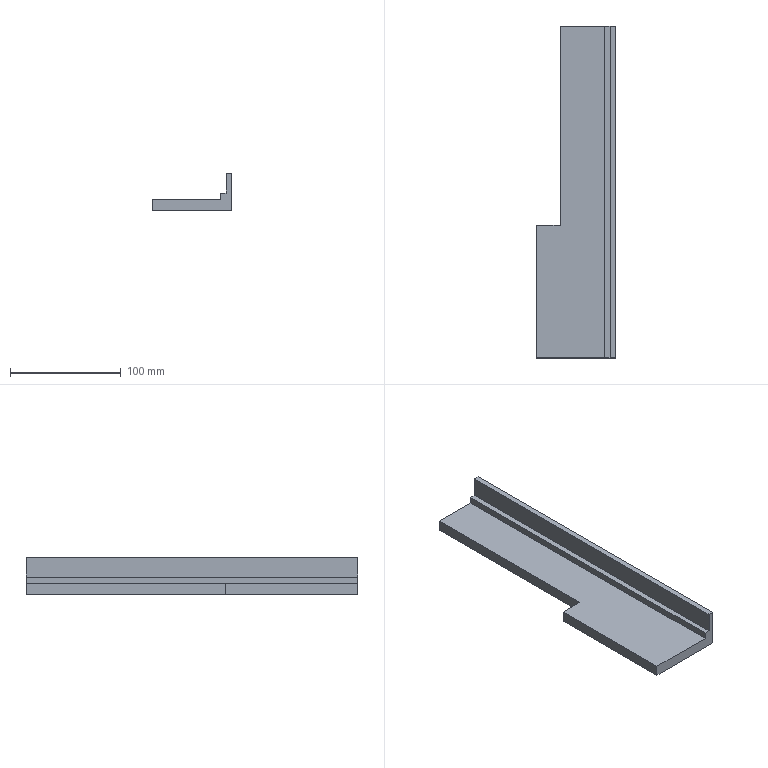Part | STEP file | Platform 1 slider plate 2 | 1 solid | 12 faces | box 71.5 x 300 x 34 mm | volume 220800 mm3 | plane 12
STEP:
#1=CARTESIAN_POINT('',(0.,150.,0.));
#2=VERTEX_POINT('',#1);
#3=CARTESIAN_POINT('',(0.,-30.,0.));
#4=VERTEX_POINT('',#3);
#5=CARTESIAN_POINT('',(0.,150.,0.));
#6=DIRECTION('',(0.,-1.,0.));
#7=VECTOR('',#6,1000.);
#8=LINE('',#5,#7);
#9=EDGE_CURVE('',#2,#4,#8,.T.);
#10=ORIENTED_EDGE('',*,*,#9,.T.);
#11=CARTESIAN_POINT('',(0.,-30.,10.));
#12=VERTEX_POINT('',#11);
#13=CARTESIAN_POINT('',(0.,-30.,-121.911));
#14=DIRECTION('',(0.,0.,1.));
#15=VECTOR('',#14,1000.);
#16=LINE('',#13,#15);
#17=EDGE_CURVE('',#4,#12,#16,.T.);
#18=ORIENTED_EDGE('',*,*,#17,.T.);
#19=CARTESIAN_POINT('',(0.,150.,10.));
#20=VERTEX_POINT('',#19);
#21=CARTESIAN_POINT('',(0.,150.,10.));
#22=DIRECTION('',(0.,-1.,0.));
#23=VECTOR('',#22,1000.);
#24=LINE('',#21,#23);
#25=EDGE_CURVE('',#20,#12,#24,.T.);
#26=ORIENTED_EDGE('',*,*,#25,.F.);
#27=CARTESIAN_POINT('',(0.,150.,10.));
#28=DIRECTION('',(0.,0.,1.));
#29=VECTOR('',#28,1000.);
#30=LINE('',#27,#29);
#31=EDGE_CURVE('',#2,#20,#30,.T.);
#32=ORIENTED_EDGE('',*,*,#31,.F.);
#33=EDGE_LOOP('',(#10,#18,#26,#32));
#34=FACE_OUTER_BOUND('',#33,.T.);
#35=CARTESIAN_POINT('',(0.,150.,10.));
#36=DIRECTION('',(1.,0.,0.));
#37=DIRECTION('',(0.,0.,-1.));
#38=AXIS2_PLACEMENT_3D('',#35,#36,#37);
#39=PLANE('',#38);
#40=ADVANCED_FACE('',(#34),#39,.F.);
#41=CARTESIAN_POINT('',(-21.5,-150.,10.));
#42=VERTEX_POINT('',#41);
#43=CARTESIAN_POINT('',(40.,-150.,10.));
#44=VERTEX_POINT('',#43);
#45=CARTESIAN_POINT('',(40.,-150.,10.));
#46=DIRECTION('',(1.,0.,0.));
#47=VECTOR('',#46,1000.);
#48=LINE('',#45,#47);
#49=EDGE_CURVE('',#42,#44,#48,.T.);
#50=ORIENTED_EDGE('',*,*,#49,.T.);
#51=CARTESIAN_POINT('',(40.,150.,10.));
#52=VERTEX_POINT('',#51);
#53=CARTESIAN_POINT('',(40.,150.,10.));
#54=DIRECTION('',(0.,-1.,0.));
#55=VECTOR('',#54,1000.);
#56=LINE('',#53,#55);
#57=EDGE_CURVE('',#52,#44,#56,.T.);
#58=ORIENTED_EDGE('',*,*,#57,.F.);
#59=CARTESIAN_POINT('',(40.,150.,10.));
#60=DIRECTION('',(1.,0.,0.));
#61=VECTOR('',#60,1000.);
#62=LINE('',#59,#61);
#63=EDGE_CURVE('',#20,#52,#62,.T.);
#64=ORIENTED_EDGE('',*,*,#63,.F.);
#65=ORIENTED_EDGE('',*,*,#25,.T.);
#66=CARTESIAN_POINT('',(-21.5,-30.,10.));
#67=VERTEX_POINT('',#66);
#68=CARTESIAN_POINT('',(0.,-30.,10.));
#69=DIRECTION('',(-1.,0.,0.));
#70=VECTOR('',#69,1000.);
#71=LINE('',#68,#70);
#72=EDGE_CURVE('',#12,#67,#71,.T.);
#73=ORIENTED_EDGE('',*,*,#72,.T.);
#74=CARTESIAN_POINT('',(-21.5,-150.,10.));
#75=DIRECTION('',(0.,-1.,0.));
#76=VECTOR('',#75,1000.);
#77=LINE('',#74,#76);
#78=EDGE_CURVE('',#67,#42,#77,.T.);
#79=ORIENTED_EDGE('',*,*,#78,.T.);
#80=EDGE_LOOP('',(#50,#58,#64,#65,#73,#79));
#81=FACE_OUTER_BOUND('',#80,.T.);
#82=CARTESIAN_POINT('',(40.,150.,10.));
#83=DIRECTION('',(0.,0.,-1.));
#84=DIRECTION('',(-1.,0.,0.));
#85=AXIS2_PLACEMENT_3D('',#82,#83,#84);
#86=PLANE('',#85);
#87=ADVANCED_FACE('',(#81),#86,.F.);
#88=CARTESIAN_POINT('',(40.,-150.,16.));
#89=VERTEX_POINT('',#88);
#90=CARTESIAN_POINT('',(40.,-150.,34.));
#91=DIRECTION('',(0.,0.,1.));
#92=VECTOR('',#91,1000.);
#93=LINE('',#90,#92);
#94=EDGE_CURVE('',#44,#89,#93,.T.);
#95=ORIENTED_EDGE('',*,*,#94,.T.);
#96=CARTESIAN_POINT('',(40.,150.,16.));
#97=VERTEX_POINT('',#96);
#98=CARTESIAN_POINT('',(40.,150.,16.));
#99=DIRECTION('',(0.,-1.,0.));
#100=VECTOR('',#99,1000.);
#101=LINE('',#98,#100);
#102=EDGE_CURVE('',#97,#89,#101,.T.);
#103=ORIENTED_EDGE('',*,*,#102,.F.);
#104=CARTESIAN_POINT('',(40.,150.,34.));
#105=DIRECTION('',(0.,0.,1.));
#106=VECTOR('',#105,1000.);
#107=LINE('',#104,#106);
#108=EDGE_CURVE('',#52,#97,#107,.T.);
#109=ORIENTED_EDGE('',*,*,#108,.F.);
#110=ORIENTED_EDGE('',*,*,#57,.T.);
#111=EDGE_LOOP('',(#95,#103,#109,#110));
#112=FACE_OUTER_BOUND('',#111,.T.);
#113=CARTESIAN_POINT('',(40.,150.,34.));
#114=DIRECTION('',(1.,0.,0.));
#115=DIRECTION('',(0.,0.,-1.));
#116=AXIS2_PLACEMENT_3D('',#113,#114,#115);
#117=PLANE('',#116);
#118=ADVANCED_FACE('',(#112),#117,.F.);
#119=CARTESIAN_POINT('',(45.,150.,34.));
#120=VERTEX_POINT('',#119);
#121=CARTESIAN_POINT('',(50.,150.,34.));
#122=VERTEX_POINT('',#121);
#123=CARTESIAN_POINT('',(50.,150.,34.));
#124=DIRECTION('',(1.,0.,0.));
#125=VECTOR('',#124,1000.);
#126=LINE('',#123,#125);
#127=EDGE_CURVE('',#120,#122,#126,.T.);
#128=ORIENTED_EDGE('',*,*,#127,.F.);
#129=CARTESIAN_POINT('',(45.,-150.,34.));
#130=VERTEX_POINT('',#129);
#131=CARTESIAN_POINT('',(45.,150.,34.));
#132=DIRECTION('',(0.,-1.,0.));
#133=VECTOR('',#132,1000.);
#134=LINE('',#131,#133);
#135=EDGE_CURVE('',#120,#130,#134,.T.);
#136=ORIENTED_EDGE('',*,*,#135,.T.);
#137=CARTESIAN_POINT('',(50.,-150.,34.));
#138=VERTEX_POINT('',#137);
#139=CARTESIAN_POINT('',(50.,-150.,34.));
#140=DIRECTION('',(1.,0.,0.));
#141=VECTOR('',#140,1000.);
#142=LINE('',#139,#141);
#143=EDGE_CURVE('',#130,#138,#142,.T.);
#144=ORIENTED_EDGE('',*,*,#143,.T.);
#145=CARTESIAN_POINT('',(50.,150.,34.));
#146=DIRECTION('',(0.,-1.,0.));
#147=VECTOR('',#146,1000.);
#148=LINE('',#145,#147);
#149=EDGE_CURVE('',#122,#138,#148,.T.);
#150=ORIENTED_EDGE('',*,*,#149,.F.);
#151=EDGE_LOOP('',(#128,#136,#144,#150));
#152=FACE_OUTER_BOUND('',#151,.T.);
#153=CARTESIAN_POINT('',(50.,150.,34.));
#154=DIRECTION('',(0.,0.,-1.));
#155=DIRECTION('',(-1.,0.,0.));
#156=AXIS2_PLACEMENT_3D('',#153,#154,#155);
#157=PLANE('',#156);
#158=ADVANCED_FACE('',(#152),#157,.F.);
#159=CARTESIAN_POINT('',(50.,-150.,0.));
#160=VERTEX_POINT('',#159);
#161=CARTESIAN_POINT('',(50.,-150.,0.));
#162=DIRECTION('',(0.,0.,-1.));
#163=VECTOR('',#162,1000.);
#164=LINE('',#161,#163);
#165=EDGE_CURVE('',#138,#160,#164,.T.);
#166=ORIENTED_EDGE('',*,*,#165,.T.);
#167=CARTESIAN_POINT('',(50.,150.,0.));
#168=VERTEX_POINT('',#167);
#169=CARTESIAN_POINT('',(50.,150.,0.));
#170=DIRECTION('',(0.,-1.,0.));
#171=VECTOR('',#170,1000.);
#172=LINE('',#169,#171);
#173=EDGE_CURVE('',#168,#160,#172,.T.);
#174=ORIENTED_EDGE('',*,*,#173,.F.);
#175=CARTESIAN_POINT('',(50.,150.,0.));
#176=DIRECTION('',(0.,0.,-1.));
#177=VECTOR('',#176,1000.);
#178=LINE('',#175,#177);
#179=EDGE_CURVE('',#122,#168,#178,.T.);
#180=ORIENTED_EDGE('',*,*,#179,.F.);
#181=ORIENTED_EDGE('',*,*,#149,.T.);
#182=EDGE_LOOP('',(#166,#174,#180,#181));
#183=FACE_OUTER_BOUND('',#182,.T.);
#184=CARTESIAN_POINT('',(50.,150.,0.));
#185=DIRECTION('',(-1.,0.,0.));
#186=DIRECTION('',(0.,0.,1.));
#187=AXIS2_PLACEMENT_3D('',#184,#185,#186);
#188=PLANE('',#187);
#189=ADVANCED_FACE('',(#183),#188,.F.);
#190=CARTESIAN_POINT('',(-21.5,-150.,0.));
#191=VERTEX_POINT('',#190);
#192=CARTESIAN_POINT('',(0.,-150.,0.));
#193=DIRECTION('',(-1.,0.,0.));
#194=VECTOR('',#193,1000.);
#195=LINE('',#192,#194);
#196=EDGE_CURVE('',#160,#191,#195,.T.);
#197=ORIENTED_EDGE('',*,*,#196,.T.);
#198=CARTESIAN_POINT('',(-21.5,-30.,0.));
#199=VERTEX_POINT('',#198);
#200=CARTESIAN_POINT('',(-21.5,-150.,0.));
#201=DIRECTION('',(0.,1.,0.));
#202=VECTOR('',#201,1000.);
#203=LINE('',#200,#202);
#204=EDGE_CURVE('',#191,#199,#203,.T.);
#205=ORIENTED_EDGE('',*,*,#204,.T.);
#206=CARTESIAN_POINT('',(0.,-30.,0.));
#207=DIRECTION('',(1.,0.,0.));
#208=VECTOR('',#207,1000.);
#209=LINE('',#206,#208);
#210=EDGE_CURVE('',#199,#4,#209,.T.);
#211=ORIENTED_EDGE('',*,*,#210,.T.);
#212=ORIENTED_EDGE('',*,*,#9,.F.);
#213=CARTESIAN_POINT('',(0.,150.,0.));
#214=DIRECTION('',(-1.,0.,0.));
#215=VECTOR('',#214,1000.);
#216=LINE('',#213,#215);
#217=EDGE_CURVE('',#168,#2,#216,.T.);
#218=ORIENTED_EDGE('',*,*,#217,.F.);
#219=ORIENTED_EDGE('',*,*,#173,.T.);
#220=EDGE_LOOP('',(#197,#205,#211,#212,#218,#219));
#221=FACE_OUTER_BOUND('',#220,.T.);
#222=CARTESIAN_POINT('',(0.,150.,0.));
#223=DIRECTION('',(0.,0.,1.));
#224=DIRECTION('',(1.,0.,0.));
#225=AXIS2_PLACEMENT_3D('',#222,#223,#224);
#226=PLANE('',#225);
#227=ADVANCED_FACE('',(#221),#226,.F.);
#228=CARTESIAN_POINT('',(45.,150.,16.));
#229=VERTEX_POINT('',#228);
#230=CARTESIAN_POINT('',(40.,150.,16.));
#231=DIRECTION('',(1.,0.,0.));
#232=VECTOR('',#231,1000.);
#233=LINE('',#230,#232);
#234=EDGE_CURVE('',#97,#229,#233,.T.);
#235=ORIENTED_EDGE('',*,*,#234,.T.);
#236=CARTESIAN_POINT('',(45.,150.,34.));
#237=DIRECTION('',(0.,0.,1.));
#238=VECTOR('',#237,1000.);
#239=LINE('',#236,#238);
#240=EDGE_CURVE('',#229,#120,#239,.T.);
#241=ORIENTED_EDGE('',*,*,#240,.T.);
#242=ORIENTED_EDGE('',*,*,#127,.T.);
#243=ORIENTED_EDGE('',*,*,#179,.T.);
#244=ORIENTED_EDGE('',*,*,#217,.T.);
#245=ORIENTED_EDGE('',*,*,#31,.T.);
#246=ORIENTED_EDGE('',*,*,#63,.T.);
#247=ORIENTED_EDGE('',*,*,#108,.T.);
#248=EDGE_LOOP('',(#235,#241,#242,#243,#244,#245,#246,#247));
#249=FACE_OUTER_BOUND('',#248,.T.);
#250=CARTESIAN_POINT('',(0.,150.,0.));
#251=DIRECTION('',(0.,-1.,0.));
#252=DIRECTION('',(0.,0.,-1.));
#253=AXIS2_PLACEMENT_3D('',#250,#251,#252);
#254=PLANE('',#253);
#255=ADVANCED_FACE('',(#249),#254,.F.);
#256=CARTESIAN_POINT('',(45.,-150.,16.));
#257=VERTEX_POINT('',#256);
#258=CARTESIAN_POINT('',(45.,-150.,34.));
#259=DIRECTION('',(0.,0.,1.));
#260=VECTOR('',#259,1000.);
#261=LINE('',#258,#260);
#262=EDGE_CURVE('',#257,#130,#261,.T.);
#263=ORIENTED_EDGE('',*,*,#262,.F.);
#264=CARTESIAN_POINT('',(40.,-150.,16.));
#265=DIRECTION('',(1.,0.,0.));
#266=VECTOR('',#265,1000.);
#267=LINE('',#264,#266);
#268=EDGE_CURVE('',#89,#257,#267,.T.);
#269=ORIENTED_EDGE('',*,*,#268,.F.);
#270=ORIENTED_EDGE('',*,*,#94,.F.);
#271=ORIENTED_EDGE('',*,*,#49,.F.);
#272=CARTESIAN_POINT('',(-21.5,-150.,-121.911));
#273=DIRECTION('',(0.,0.,1.));
#274=VECTOR('',#273,1000.);
#275=LINE('',#272,#274);
#276=EDGE_CURVE('',#191,#42,#275,.T.);
#277=ORIENTED_EDGE('',*,*,#276,.F.);
#278=ORIENTED_EDGE('',*,*,#196,.F.);
#279=ORIENTED_EDGE('',*,*,#165,.F.);
#280=ORIENTED_EDGE('',*,*,#143,.F.);
#281=EDGE_LOOP('',(#263,#269,#270,#271,#277,#278,#279,#280));
#282=FACE_OUTER_BOUND('',#281,.T.);
#283=CARTESIAN_POINT('',(0.,-150.,0.));
#284=DIRECTION('',(0.,-1.,0.));
#285=DIRECTION('',(0.,0.,-1.));
#286=AXIS2_PLACEMENT_3D('',#283,#284,#285);
#287=PLANE('',#286);
#288=ADVANCED_FACE('',(#282),#287,.T.);
#289=ORIENTED_EDGE('',*,*,#262,.T.);
#290=ORIENTED_EDGE('',*,*,#135,.F.);
#291=ORIENTED_EDGE('',*,*,#240,.F.);
#292=CARTESIAN_POINT('',(45.,150.,16.));
#293=DIRECTION('',(0.,-1.,0.));
#294=VECTOR('',#293,1000.);
#295=LINE('',#292,#294);
#296=EDGE_CURVE('',#229,#257,#295,.T.);
#297=ORIENTED_EDGE('',*,*,#296,.T.);
#298=EDGE_LOOP('',(#289,#290,#291,#297));
#299=FACE_OUTER_BOUND('',#298,.T.);
#300=CARTESIAN_POINT('',(45.,150.,34.));
#301=DIRECTION('',(1.,0.,0.));
#302=DIRECTION('',(0.,0.,-1.));
#303=AXIS2_PLACEMENT_3D('',#300,#301,#302);
#304=PLANE('',#303);
#305=ADVANCED_FACE('',(#299),#304,.F.);
#306=ORIENTED_EDGE('',*,*,#268,.T.);
#307=ORIENTED_EDGE('',*,*,#296,.F.);
#308=ORIENTED_EDGE('',*,*,#234,.F.);
#309=ORIENTED_EDGE('',*,*,#102,.T.);
#310=EDGE_LOOP('',(#306,#307,#308,#309));
#311=FACE_OUTER_BOUND('',#310,.T.);
#312=CARTESIAN_POINT('',(40.,150.,16.));
#313=DIRECTION('',(0.,0.,-1.));
#314=DIRECTION('',(-1.,0.,0.));
#315=AXIS2_PLACEMENT_3D('',#312,#313,#314);
#316=PLANE('',#315);
#317=ADVANCED_FACE('',(#311),#316,.F.);
#318=ORIENTED_EDGE('',*,*,#204,.F.);
#319=ORIENTED_EDGE('',*,*,#276,.T.);
#320=ORIENTED_EDGE('',*,*,#78,.F.);
#321=CARTESIAN_POINT('',(-21.5,-30.,-121.911));
#322=DIRECTION('',(0.,0.,1.));
#323=VECTOR('',#322,1000.);
#324=LINE('',#321,#323);
#325=EDGE_CURVE('',#199,#67,#324,.T.);
#326=ORIENTED_EDGE('',*,*,#325,.F.);
#327=EDGE_LOOP('',(#318,#319,#320,#326));
#328=FACE_OUTER_BOUND('',#327,.T.);
#329=CARTESIAN_POINT('',(-21.5,-150.,-121.911));
#330=DIRECTION('',(-1.,0.,0.));
#331=DIRECTION('',(0.,0.,1.));
#332=AXIS2_PLACEMENT_3D('',#329,#330,#331);
#333=PLANE('',#332);
#334=ADVANCED_FACE('',(#328),#333,.T.);
#335=ORIENTED_EDGE('',*,*,#210,.F.);
#336=ORIENTED_EDGE('',*,*,#325,.T.);
#337=ORIENTED_EDGE('',*,*,#72,.F.);
#338=ORIENTED_EDGE('',*,*,#17,.F.);
#339=EDGE_LOOP('',(#335,#336,#337,#338));
#340=FACE_OUTER_BOUND('',#339,.T.);
#341=CARTESIAN_POINT('',(0.,-30.,-121.911));
#342=DIRECTION('',(0.,1.,0.));
#343=DIRECTION('',(0.,0.,1.));
#344=AXIS2_PLACEMENT_3D('',#341,#342,#343);
#345=PLANE('',#344);
#346=ADVANCED_FACE('',(#340),#345,.T.);
#347=CLOSED_SHELL('',(#40,#87,#118,#158,#189,#227,#255,#288,#305,#317,#334,#346));
#348=MANIFOLD_SOLID_BREP('',#347);
#349=CARTESIAN_POINT('',(0.,0.,0.));
#350=DIRECTION('',(0.,0.,1.));
#351=DIRECTION('',(1.,0.,0.));
#352=AXIS2_PLACEMENT_3D('',#349,#350,#351);
#353=(LENGTH_UNIT()NAMED_UNIT(*)SI_UNIT(.MILLI.,.METRE.));
#354=UNCERTAINTY_MEASURE_WITH_UNIT(LENGTH_MEASURE(0.00001),#353,'','');
#355=(NAMED_UNIT(*)PLANE_ANGLE_UNIT()SI_UNIT($,.RADIAN.));
#356=(NAMED_UNIT(*)SI_UNIT($,.STERADIAN.)SOLID_ANGLE_UNIT());
#357=(GEOMETRIC_REPRESENTATION_CONTEXT(3)GLOBAL_UNCERTAINTY_ASSIGNED_CONTEXT((#354))GLOBAL_UNIT_ASSIGNED_CONTEXT((#353,#355,#356))REPRESENTATION_CONTEXT('',''));
#358=ADVANCED_BREP_SHAPE_REPRESENTATION('',(#348,#352),#357);